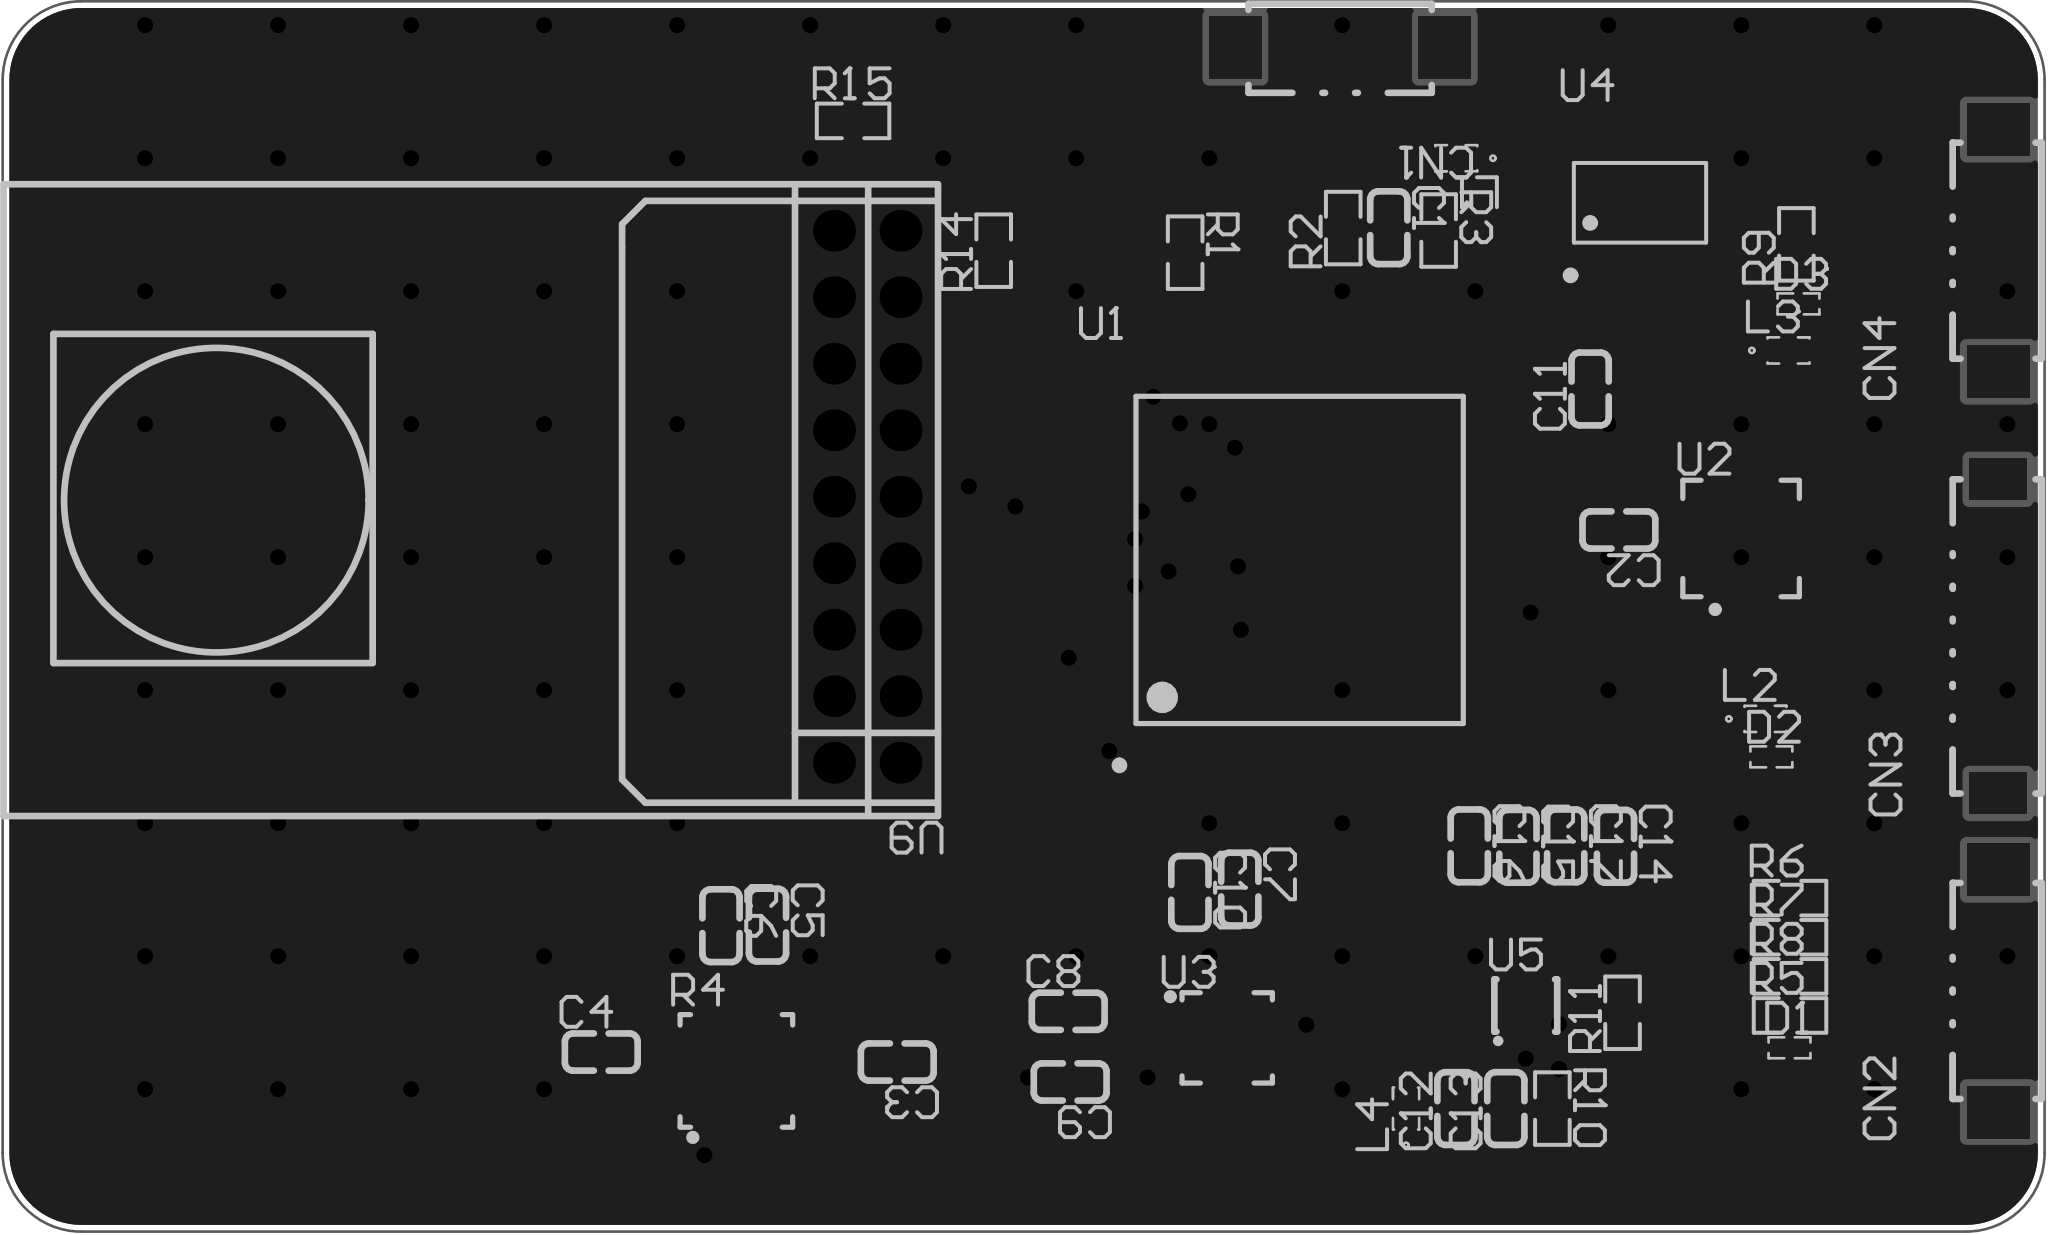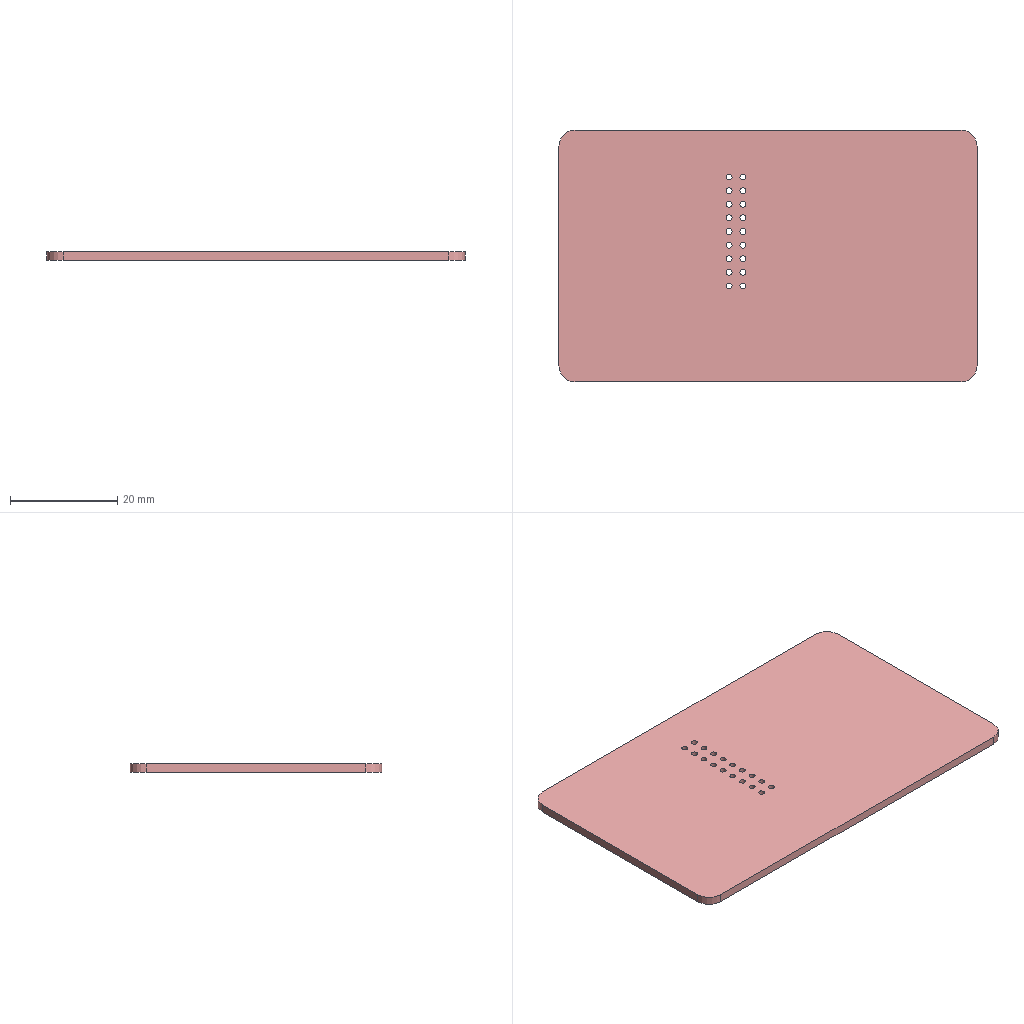Circuit board layout | Altium Designer | box 78 x 47 x 1.6 mm
Layer stack:
# Altium Designer layer stack of  (unit mm; dielectric type: 0 none, 1 core, 2 prepreg, 3 surface material)
index,name,kind,layer,copper_thickness_mm,dielectric_type,dielectric_thickness_mm,dielectric_material,dielectric_constant
0,Top Paste Mask Layer,other,,,,,,
1,Top Silkscreen Layer,other,,,,,,
2,Top Solder Mask Layer,dielectric,,,3,0.01,,3.3
3,Top Layer,copper,Top Layer,0.035,,,,
4,Dielectric1,dielectric,,,3,1.51,FR4,4.5
5,Bottom Layer,copper,Bottom Layer,0.035,,,,
6,Bottom Solder Mask Layer,dielectric,,,3,0.01,,3.3
7,Bottom Silkscreen Layer,other,,,,,,
8,Bottom Paste Mask Layer,other,,,,,,
# drill layer pairs: low layer,high layer
drill_pair,Top Layer,Bottom Layer
Part placement:
Designator,Comment,Layer,Footprint,Center-X(mm),Center-Y(mm),Rotation
C1,100nF,TopLayer,C0603,138.023,124.067,270
C2,10nF,TopLayer,C0603,146.812,112.522,180
C3,2U2,TopLayer,C0603,119.253,92.202,180
C4,2U2,TopLayer,C0603,107.95,92.583,0
C5,2U2,TopLayer,C0603,114.298,97.432,270
C6,0U1,TopLayer,C0603,112.522,97.409,270
C7,10UF,TopLayer,C0603,132.334,98.806,270
C8,10UF,TopLayer,C0603,125.782,94.139,0
C9,10UF,TopLayer,C0603,125.857,91.44,180
C10,10UF,TopLayer,C0603,130.429,98.679,270
C11,100nF,TopLayer,C0603,145.713,117.908,90
C12,100nF,TopLayer,C0603,140.589,90.424,90
C13,100nF,TopLayer,C0603,142.494,90.424,90
C14,100nF,TopLayer,C0603,146.681,100.441,270
C15,100nF,TopLayer,C0603,142.955,100.441,270
C16,100nF,TopLayer,C0603,141.097,100.457,270
C17,100nF,TopLayer,C0603,144.78,100.457,270
CN1,DF13C-3P-1.25V(51),TopLayer,CONN-SMD_3P-P1.25_DF13C-3P-1.25V,136.165,129.601,180
CN2,DF13C-4P-1.25V(51),TopLayer,CONN-SMD_4P-P1.25_DF13C-4P-1.25V,159.94,94.916,90
CN3,DF13C-7P-1.25V(51),TopLayer,CONN-SMD_7P-P1.25_DF13C-7P-1.25V,159.94,108.458,90
CN4,DF13C-4P-1.25V(51),TopLayer,CONN-SMD_4P-P1.25_DF13C-4P-1.25V,159.94,123.19,90
D1,PESD0402-05ST-ES,TopLayer,DFN1006-2L-BI,153.327,92.746,0
D2,PESD0402-05ST-ES,TopLayer,DFN1006-2L-BI,152.635,103.858,0
D3,PESD0402-05ST-ES,TopLayer,DFN1006-2L-BI,153.67,121.158,0
L1,KNH16C104DA5TS,TopLayer,FILTER-SMD_3P-L1.6-W0.8_YFF18PCXXXXXXX,140.602,126.722,180
L2,KNH16C104DA5TS,TopLayer,FILTER-SMD_3P-L1.6-W0.8_YFF18PCXXXXXXX,152.409,105.307,0
L3,KNH16C104DA5TS,TopLayer,FILTER-SMD_3P-L1.6-W0.8_YFF18PCXXXXXXX,153.289,119.38,0
L4,KNH16C104DA5TS,TopLayer,FILTER-SMD_3P-L1.6-W0.8_YFF18PCXXXXXXX,138.684,90.424,90
R1,10K,TopLayer,R0603,130.248,123.114,270
R2,10K,TopLayer,R0603,136.284,124.055,90
R3,10K,TopLayer,R0603,139.928,123.96,270
R4,MPU-6000,TopLayer,QFN-24_L4.0-W4.0-P0.50-BL-EP2.7,113.097,91.862,0
R5,120R,TopLayer,R0603,153.347,93.98,0
R6,120R,TopLayer,R0603,153.347,98.461,0
R7,120R,TopLayer,R0603,153.347,96.967,0
R8,120R,TopLayer,R0603,153.347,95.474,0
R9,120R,TopLayer,R0603,153.59,123.431,90
R10,120R,TopLayer,R0603,144.272,90.424,270
R11,10K,TopLayer,R0603,146.951,94.084,90
R14,10K,TopLayer,R0603,122.936,123.19,90
R15,10K,TopLayer,R0603,117.566,128.147,0
U1,STM32F427VGT6,TopLayer,LQFP-100_L14.0-W14.0-P0.50-LS16.0-BL,134.62,111.379,0
U2,L3GD20,TopLayer,LGA-16_L4.0-W4.0-P0.65-BL,151.478,112.198,0
U3,LSM303D,TopLayer,LGA-16_L3.0-W3.0-P0.50-TL,131.854,93.123,0
U4,MAX3051ESA+T,TopLayer,SOIC-8_L4.9-W3.9-P1.27-LS6.0-BL,147.618,125.02,0
U5,MIC5332-PPYMT-TR,TopLayer,MLF-8_L2.0-W2.0-P0.50-BL-EP,143.256,94.361,0
U9,OV2640 Camera Board,TopLayer,SENSORM-TH_L35.7-W3.9-OV2640,118.11,113.792,180
Pad and via stacks:
# Altium Designer via and pad stacks of  (unit mm). Each distinct definition once, with the count of objects using it.
# via: kind,start_layer,end_layer,hole_mm,diameter_mm,mode(0 simple;1 top-mid-bottom;2 full stack),diameter_per_layer,count,example_net
# pad: kind,layer,hole_mm,hole_type(0 round;1 square;2 slot),plating,top_size,top_shape(1 round;2 rect;3 octagon;9 rounded rect),mid_size,bottom_size,mode,footprint,size_per_layer,count,example
pad,Top Layer,0,0,plated,0.8x0.9,2,0.8x0.9,0.8x0.9,0,C0603,,34,C1.2
pad,Top Layer,0,0,plated,2x0.7,2,2x0.7,2x0.7,0,CONN-SMD_3P-P1.25_DF13C-3P-1.25V,,3,CN1.1
pad,Top Layer,0,0,plated,2x2.4,2,2x2.4,2x2.4,0,CONN-SMD_3P-P1.25_DF13C-3P-1.25V,,2,CN1.5
pad,Top Layer,0,0,plated,1.8x0.7,2,1.8x0.7,1.8x0.7,0,CONN-SMD_4P-P1.25_DF13C-4P-1.25V,,8,CN2.1
pad,Top Layer,0,0,plated,2x2.4,2,2x2.4,2x2.4,0,CONN-SMD_4P-P1.25_DF13C-4P-1.25V,,4,CN2.6
pad,Top Layer,0,0,plated,1.8x0.7,2,1.8x0.7,1.8x0.7,0,CONN-SMD_7P-P1.25_DF13C-7P-1.25V,,7,CN3.1
pad,Top Layer,0,0,plated,1.6x2.2,2,1.6x2.2,1.6x2.2,0,CONN-SMD_7P-P1.25_DF13C-7P-1.25V,,2,CN3.9
pad,Top Layer,0,0,plated,0.55x0.6,2,0.55x0.6,0.55x0.6,0,DFN1006-2L-BI,,6,D1.1
pad,Top Layer,0,0,plated,0.6x0.6,2,0.6x0.6,0.6x0.6,0,FILTER-SMD_3P-L1.6-W0.8_YFF18PCXXXXXXX,,8,L1.1
pad,Top Layer,0,0,plated,0.4x0.4,2,0.4x0.4,0.4x0.4,0,FILTER-SMD_3P-L1.6-W0.8_YFF18PCXXXXXXX,,8,L1.2
pad,Top Layer,0,0,plated,0.8065x0.864,2,0.8065x0.864,0.8065x0.864,0,R0603,,24,R1.2
pad,Top Layer,0,0,plated,0.28x0.8,1,0.28x0.8,0.28x0.8,0,QFN-24_L4.0-W4.0-P0.50-BL-EP2.7,,12,R4.1
pad,Top Layer,0,0,plated,0.8x0.28,1,0.8x0.28,0.8x0.28,0,QFN-24_L4.0-W4.0-P0.50-BL-EP2.7,,12,R4.7
pad,Top Layer,0,0,plated,2.7x2.7,2,2.7x2.7,2.7x2.7,0,QFN-24_L4.0-W4.0-P0.50-BL-EP2.7,,1,R4.25
pad,Top Layer,0,0,plated,1.6x0.3,1,1.6x0.3,1.6x0.3,0,LQFP-100_L14.0-W14.0-P0.50-LS16.0-BL,,50,U1.100
pad,Top Layer,0,0,plated,0.3x1.6,1,0.3x1.6,0.3x1.6,0,LQFP-100_L14.0-W14.0-P0.50-LS16.0-BL,,50,U1.75
pad,Top Layer,0,0,plated,0.4x0.9,1,0.4x0.9,0.4x0.9,0,LGA-16_L4.0-W4.0-P0.65-BL,,16,U2.16
pad,Top Layer,0,0,plated,0.8x0.28,1,0.8x0.28,0.8x0.28,0,LGA-16_L3.0-W3.0-P0.50-TL,,10,U3.1
pad,Top Layer,0,0,plated,0.28x0.8,1,0.28x0.8,0.28x0.8,0,LGA-16_L3.0-W3.0-P0.50-TL,,6,U3.6
pad,Top Layer,0,0,plated,0.588x2.045,1,0.588x2.045,0.588x2.045,0,SOIC-8_L4.9-W3.9-P1.27-LS6.0-BL,,8,U4.1
pad,Top Layer,0,0,plated,0.25x0.6,2,0.25x0.6,0.25x0.6,0,MLF-8_L2.0-W2.0-P0.50-BL-EP,,8,U5.1
pad,Top Layer,0,0,plated,1.2x0.6,2,1.2x0.6,1.2x0.6,0,MLF-8_L2.0-W2.0-P0.50-BL-EP,,1,U5.9
pad,Multi-Layer,1.1,0,plated,1.6x1.6,1,1.6x1.6,1.6x1.6,0,SENSORM-TH_L35.7-W3.9-OV2640,,18,U9.1
via,Top Layer,Bottom Layer,0.3048,0.61,0,,113,$1N6097
Copper pours:
name,layer,net,type(0 solid;1 hatched;2 none)
Top Layer-GND,Top Layer,GND,0
Bottom Layer-GND,Bottom Layer,GND,0